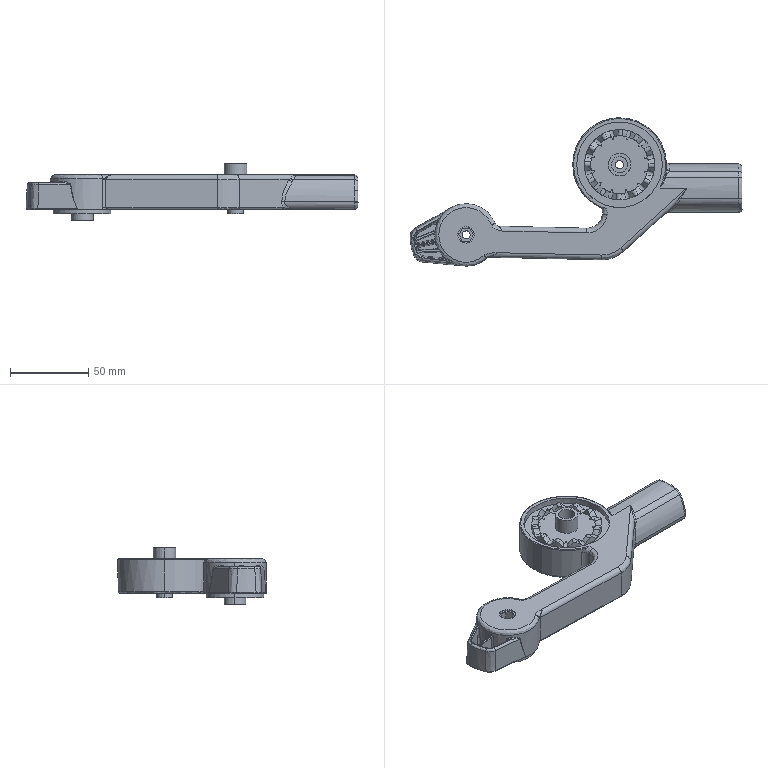Part | SolidWorks | features BaseBody 1 | 1 solid | 652 faces | box 212.741 x 95 x 36 mm | volume 90417 mm3 | plane 300 | cylinder 174 | spline 171 | torus 4 | cone 3 | commonest cylinder face diameters 37 x15 1 x13 2 x10 54 x10 4 x9 46 x7